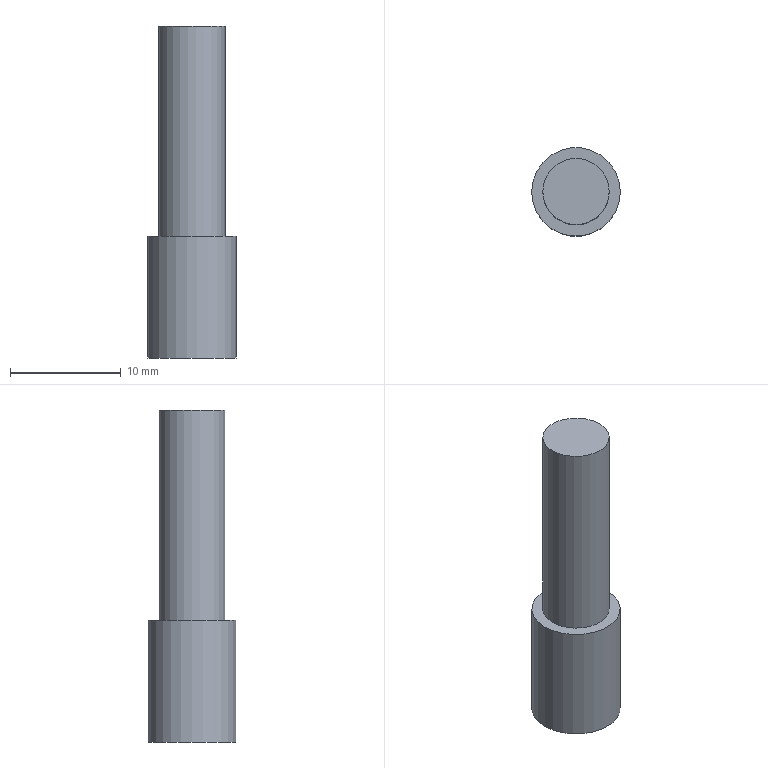Part | NX | features solid 2 | 1 solid | 5 faces | box 8 x 8 x 30 mm | volume 1090 mm3 | plane 3 | cylinder 2 | commonest cylinder face diameters 6 x1 8 x1
STEP:
#1=CARTESIAN_POINT('',(70.,72.,-20.));
#2=VERTEX_POINT('',#1);
#3=CARTESIAN_POINT('',(67.,72.,-20.));
#4=DIRECTION('',(0.,0.,1.));
#5=DIRECTION('',(1.,0.,0.));
#6=AXIS2_PLACEMENT_3D('',#3,#4,#5);
#7=CIRCLE('',#6,3.);
#8=EDGE_CURVE('',#2,#2,#7,.T.);
#9=ORIENTED_EDGE('',*,*,#8,.F.);
#10=EDGE_LOOP('',(#9));
#11=FACE_BOUND('',#10,.T.);
#12=CARTESIAN_POINT('',(64.,72.,-39.));
#13=VERTEX_POINT('',#12);
#14=CARTESIAN_POINT('',(67.,72.,-39.));
#15=DIRECTION('',(0.,0.,-1.));
#16=DIRECTION('',(-1.,0.,0.));
#17=AXIS2_PLACEMENT_3D('',#14,#15,#16);
#18=CIRCLE('',#17,3.);
#19=EDGE_CURVE('',#13,#13,#18,.F.);
#20=ORIENTED_EDGE('',*,*,#19,.T.);
#21=EDGE_LOOP('',(#20));
#22=FACE_BOUND('',#21,.T.);
#23=CARTESIAN_POINT('',(67.,72.,-35.));
#24=DIRECTION('',(0.,0.,1.));
#25=DIRECTION('',(1.,0.,0.));
#26=AXIS2_PLACEMENT_3D('',#23,#24,#25);
#27=CYLINDRICAL_SURFACE('',#26,3.);
#28=ADVANCED_FACE('',(#11,#22),#27,.T.);
#29=ORIENTED_EDGE('',*,*,#8,.T.);
#30=EDGE_LOOP('',(#29));
#31=FACE_BOUND('',#30,.T.);
#32=CARTESIAN_POINT('',(67.,72.,-20.));
#33=DIRECTION('',(0.,0.,1.));
#34=DIRECTION('',(1.,0.,0.));
#35=AXIS2_PLACEMENT_3D('',#32,#33,#34);
#36=PLANE('',#35);
#37=ADVANCED_FACE('',(#31),#36,.T.);
#38=CARTESIAN_POINT('',(63.,72.,-39.));
#39=VERTEX_POINT('',#38);
#40=CARTESIAN_POINT('',(67.,72.,-39.));
#41=DIRECTION('',(0.,0.,-1.));
#42=DIRECTION('',(-1.,0.,0.));
#43=AXIS2_PLACEMENT_3D('',#40,#41,#42);
#44=CIRCLE('',#43,4.);
#45=EDGE_CURVE('',#39,#39,#44,.T.);
#46=ORIENTED_EDGE('',*,*,#45,.T.);
#47=EDGE_LOOP('',(#46));
#48=FACE_BOUND('',#47,.T.);
#49=CARTESIAN_POINT('',(63.,72.,-50.));
#50=VERTEX_POINT('',#49);
#51=CARTESIAN_POINT('',(67.,72.,-50.));
#52=DIRECTION('',(0.,0.,-1.));
#53=DIRECTION('',(-1.,0.,0.));
#54=AXIS2_PLACEMENT_3D('',#51,#52,#53);
#55=CIRCLE('',#54,4.);
#56=EDGE_CURVE('',#50,#50,#55,.T.);
#57=ORIENTED_EDGE('',*,*,#56,.F.);
#58=EDGE_LOOP('',(#57));
#59=FACE_BOUND('',#58,.T.);
#60=CARTESIAN_POINT('',(67.,72.,-38.));
#61=DIRECTION('',(0.,0.,-1.));
#62=DIRECTION('',(-1.,0.,0.));
#63=AXIS2_PLACEMENT_3D('',#60,#61,#62);
#64=CYLINDRICAL_SURFACE('',#63,4.);
#65=ADVANCED_FACE('',(#48,#59),#64,.T.);
#66=ORIENTED_EDGE('',*,*,#19,.F.);
#67=EDGE_LOOP('',(#66));
#68=FACE_BOUND('',#67,.T.);
#69=ORIENTED_EDGE('',*,*,#45,.F.);
#70=EDGE_LOOP('',(#69));
#71=FACE_BOUND('',#70,.T.);
#72=CARTESIAN_POINT('',(67.,72.,-39.));
#73=DIRECTION('',(0.,0.,-1.));
#74=DIRECTION('',(-1.,0.,0.));
#75=AXIS2_PLACEMENT_3D('',#72,#73,#74);
#76=PLANE('',#75);
#77=ADVANCED_FACE('',(#68,#71),#76,.F.);
#78=ORIENTED_EDGE('',*,*,#56,.T.);
#79=EDGE_LOOP('',(#78));
#80=FACE_BOUND('',#79,.T.);
#81=CARTESIAN_POINT('',(8.802,-49.836,-50.));
#82=DIRECTION('',(0.,0.,1.));
#83=DIRECTION('',(-1.,0.,0.));
#84=AXIS2_PLACEMENT_3D('',#81,#82,#83);
#85=PLANE('',#84);
#86=ADVANCED_FACE('',(#80),#85,.F.);
#87=CLOSED_SHELL('',(#28,#37,#65,#77,#86));
#88=MANIFOLD_SOLID_BREP('',#87);
#89=(LENGTH_UNIT()NAMED_UNIT(*)SI_UNIT(.MILLI.,.METRE.));
#90=UNCERTAINTY_MEASURE_WITH_UNIT(LENGTH_MEASURE(0.00001),#89,'','');
#91=(NAMED_UNIT(*)PLANE_ANGLE_UNIT()SI_UNIT($,.RADIAN.));
#92=(NAMED_UNIT(*)SI_UNIT($,.STERADIAN.)SOLID_ANGLE_UNIT());
#93=(GEOMETRIC_REPRESENTATION_CONTEXT(3)GLOBAL_UNCERTAINTY_ASSIGNED_CONTEXT((#90))GLOBAL_UNIT_ASSIGNED_CONTEXT((#89,#91,#92))REPRESENTATION_CONTEXT('',''));
#94=ADVANCED_BREP_SHAPE_REPRESENTATION('',(#88),#93);